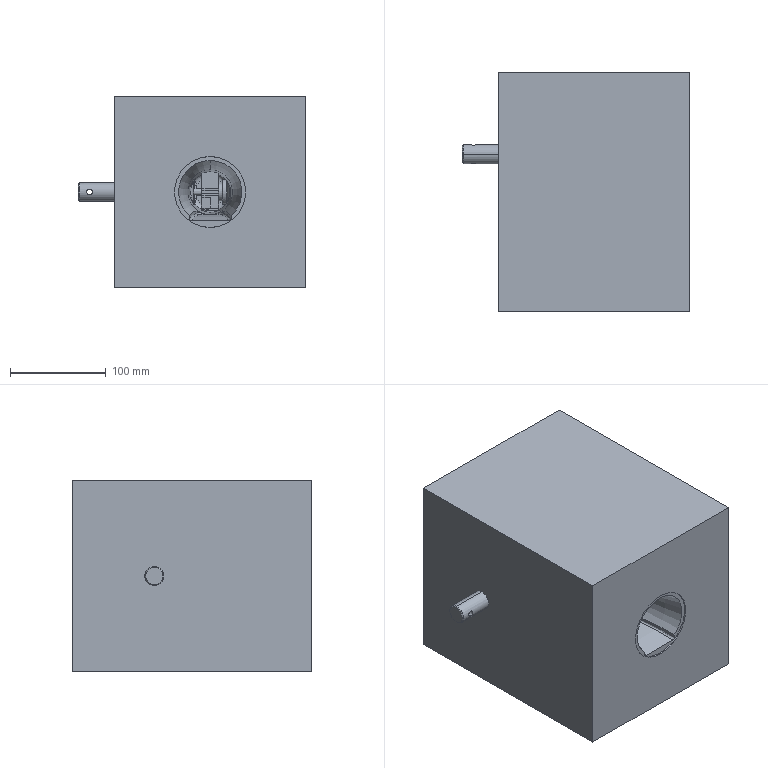Part | STEP file | Cavity - Tower - 1 cav - Insert 2 | 2 solids | 104 faces | box 238 x 250 x 200 mm | volume 9720749 mm3 | plane 43 | spline 20 | cylinder 17 | cone 13 | torus 9 | sphere 2 | commonest cylinder face diameters 20 x6 1.018 x2 6 x2 6.105 x2 20.711 x2 28.622 x2